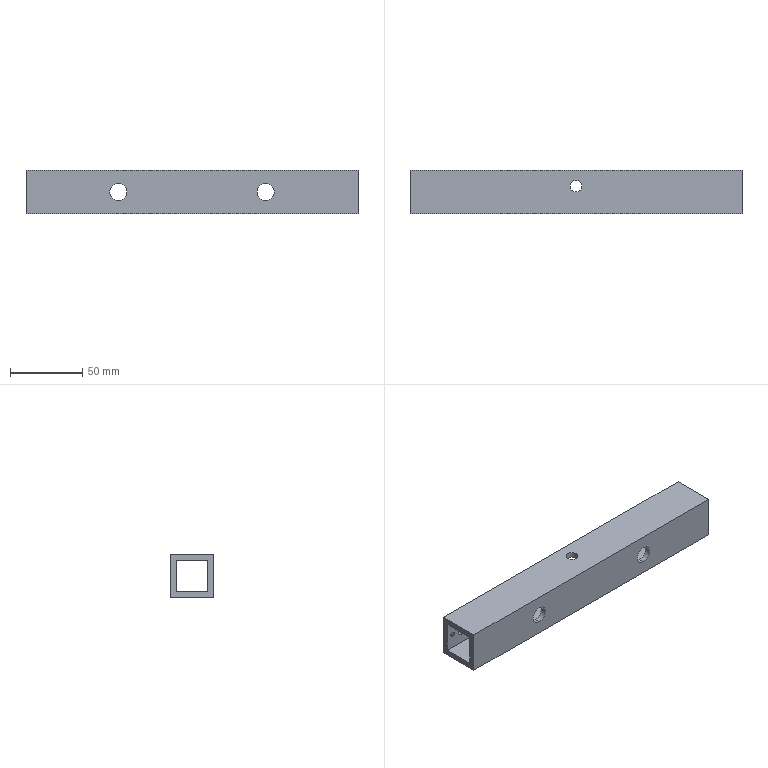Part | STEP file | Blade fixing rod | 1 solid | 37 faces | box 230 x 30 x 30 mm | volume 83181 mm3 | cylinder 24 | plane 13 | commonest cylinder face diameters 3.3 x8 4 x4 8 x4 9 x4 12 x4
STEP:
#1=CARTESIAN_POINT('',(-51.,4.,7.318));
#2=VERTEX_POINT('',#1);
#3=CARTESIAN_POINT('',(-51.,4.,-4.682));
#4=VERTEX_POINT('',#3);
#5=CARTESIAN_POINT('',(-51.,4.,1.318));
#6=DIRECTION('',(0.,-1.,0.));
#7=DIRECTION('',(0.,0.,-1.));
#8=AXIS2_PLACEMENT_3D('',#5,#6,#7);
#9=CIRCLE('',#8,6.);
#10=EDGE_CURVE('',#2,#4,#9,.T.);
#11=ORIENTED_EDGE('',*,*,#10,.F.);
#12=CARTESIAN_POINT('',(-51.,0.,7.318));
#13=VERTEX_POINT('',#12);
#14=CARTESIAN_POINT('',(-51.,0.,7.318));
#15=DIRECTION('',(0.,-1.,0.));
#16=VECTOR('',#15,1000.);
#17=LINE('',#14,#16);
#18=EDGE_CURVE('',#2,#13,#17,.T.);
#19=ORIENTED_EDGE('',*,*,#18,.T.);
#20=CARTESIAN_POINT('',(-51.,0.,-4.682));
#21=VERTEX_POINT('',#20);
#22=CARTESIAN_POINT('',(-51.,0.,1.318));
#23=DIRECTION('',(0.,-1.,0.));
#24=DIRECTION('',(0.,0.,-1.));
#25=AXIS2_PLACEMENT_3D('',#22,#23,#24);
#26=CIRCLE('',#25,6.);
#27=EDGE_CURVE('',#13,#21,#26,.T.);
#28=ORIENTED_EDGE('',*,*,#27,.T.);
#29=CARTESIAN_POINT('',(-51.,0.,-4.682));
#30=DIRECTION('',(0.,-1.,0.));
#31=VECTOR('',#30,1000.);
#32=LINE('',#29,#31);
#33=EDGE_CURVE('',#4,#21,#32,.T.);
#34=ORIENTED_EDGE('',*,*,#33,.F.);
#35=EDGE_LOOP('',(#11,#19,#28,#34));
#36=FACE_OUTER_BOUND('',#35,.T.);
#37=CARTESIAN_POINT('',(-51.,0.,1.318));
#38=DIRECTION('',(0.,-1.,0.));
#39=DIRECTION('',(0.,0.,-1.));
#40=AXIS2_PLACEMENT_3D('',#37,#38,#39);
#41=CYLINDRICAL_SURFACE('',#40,6.);
#42=ADVANCED_FACE('',(#36),#41,.F.);
#43=CARTESIAN_POINT('',(51.,4.,7.318));
#44=VERTEX_POINT('',#43);
#45=CARTESIAN_POINT('',(51.,4.,-4.682));
#46=VERTEX_POINT('',#45);
#47=CARTESIAN_POINT('',(51.,4.,1.318));
#48=DIRECTION('',(0.,-1.,0.));
#49=DIRECTION('',(0.,0.,-1.));
#50=AXIS2_PLACEMENT_3D('',#47,#48,#49);
#51=CIRCLE('',#50,6.);
#52=EDGE_CURVE('',#44,#46,#51,.T.);
#53=ORIENTED_EDGE('',*,*,#52,.F.);
#54=CARTESIAN_POINT('',(51.,0.,7.318));
#55=VERTEX_POINT('',#54);
#56=CARTESIAN_POINT('',(51.,0.,7.318));
#57=DIRECTION('',(0.,-1.,0.));
#58=VECTOR('',#57,1000.);
#59=LINE('',#56,#58);
#60=EDGE_CURVE('',#44,#55,#59,.T.);
#61=ORIENTED_EDGE('',*,*,#60,.T.);
#62=CARTESIAN_POINT('',(51.,0.,-4.682));
#63=VERTEX_POINT('',#62);
#64=CARTESIAN_POINT('',(51.,0.,1.318));
#65=DIRECTION('',(0.,-1.,0.));
#66=DIRECTION('',(0.,0.,-1.));
#67=AXIS2_PLACEMENT_3D('',#64,#65,#66);
#68=CIRCLE('',#67,6.);
#69=EDGE_CURVE('',#55,#63,#68,.T.);
#70=ORIENTED_EDGE('',*,*,#69,.T.);
#71=CARTESIAN_POINT('',(51.,0.,-4.682));
#72=DIRECTION('',(0.,-1.,0.));
#73=VECTOR('',#72,1000.);
#74=LINE('',#71,#73);
#75=EDGE_CURVE('',#46,#63,#74,.T.);
#76=ORIENTED_EDGE('',*,*,#75,.F.);
#77=EDGE_LOOP('',(#53,#61,#70,#76));
#78=FACE_OUTER_BOUND('',#77,.T.);
#79=CARTESIAN_POINT('',(51.,0.,1.318));
#80=DIRECTION('',(0.,-1.,0.));
#81=DIRECTION('',(0.,0.,-1.));
#82=AXIS2_PLACEMENT_3D('',#79,#80,#81);
#83=CYLINDRICAL_SURFACE('',#82,6.);
#84=ADVANCED_FACE('',(#78),#83,.F.);
#85=CARTESIAN_POINT('',(110.,26.,-0.3322));
#86=VERTEX_POINT('',#85);
#87=CARTESIAN_POINT('',(110.,26.,2.968));
#88=VERTEX_POINT('',#87);
#89=CARTESIAN_POINT('',(110.,26.,1.318));
#90=DIRECTION('',(0.,1.,0.));
#91=DIRECTION('',(0.,0.,1.));
#92=AXIS2_PLACEMENT_3D('',#89,#90,#91);
#93=CIRCLE('',#92,1.65);
#94=EDGE_CURVE('',#86,#88,#93,.T.);
#95=ORIENTED_EDGE('',*,*,#94,.F.);
#96=CARTESIAN_POINT('',(110.,30.,-0.3322));
#97=VERTEX_POINT('',#96);
#98=CARTESIAN_POINT('',(110.,30.,-0.3322));
#99=DIRECTION('',(0.,1.,0.));
#100=VECTOR('',#99,1000.);
#101=LINE('',#98,#100);
#102=EDGE_CURVE('',#86,#97,#101,.T.);
#103=ORIENTED_EDGE('',*,*,#102,.T.);
#104=CARTESIAN_POINT('',(110.,30.,2.968));
#105=VERTEX_POINT('',#104);
#106=CARTESIAN_POINT('',(110.,30.,1.318));
#107=DIRECTION('',(0.,1.,0.));
#108=DIRECTION('',(0.,0.,1.));
#109=AXIS2_PLACEMENT_3D('',#106,#107,#108);
#110=CIRCLE('',#109,1.65);
#111=EDGE_CURVE('',#97,#105,#110,.T.);
#112=ORIENTED_EDGE('',*,*,#111,.T.);
#113=CARTESIAN_POINT('',(110.,30.,2.968));
#114=DIRECTION('',(0.,1.,0.));
#115=VECTOR('',#114,1000.);
#116=LINE('',#113,#115);
#117=EDGE_CURVE('',#88,#105,#116,.T.);
#118=ORIENTED_EDGE('',*,*,#117,.F.);
#119=EDGE_LOOP('',(#95,#103,#112,#118));
#120=FACE_OUTER_BOUND('',#119,.T.);
#121=CARTESIAN_POINT('',(110.,30.,1.318));
#122=DIRECTION('',(0.,1.,0.));
#123=DIRECTION('',(0.,0.,1.));
#124=AXIS2_PLACEMENT_3D('',#121,#122,#123);
#125=CYLINDRICAL_SURFACE('',#124,1.65);
#126=ADVANCED_FACE('',(#120),#125,.F.);
#127=CARTESIAN_POINT('',(90.,26.,-0.3322));
#128=VERTEX_POINT('',#127);
#129=CARTESIAN_POINT('',(90.,26.,2.968));
#130=VERTEX_POINT('',#129);
#131=CARTESIAN_POINT('',(90.,26.,1.318));
#132=DIRECTION('',(0.,1.,0.));
#133=DIRECTION('',(0.,0.,1.));
#134=AXIS2_PLACEMENT_3D('',#131,#132,#133);
#135=CIRCLE('',#134,1.65);
#136=EDGE_CURVE('',#128,#130,#135,.T.);
#137=ORIENTED_EDGE('',*,*,#136,.F.);
#138=CARTESIAN_POINT('',(90.,30.,-0.3322));
#139=VERTEX_POINT('',#138);
#140=CARTESIAN_POINT('',(90.,30.,-0.3322));
#141=DIRECTION('',(0.,1.,0.));
#142=VECTOR('',#141,1000.);
#143=LINE('',#140,#142);
#144=EDGE_CURVE('',#128,#139,#143,.T.);
#145=ORIENTED_EDGE('',*,*,#144,.T.);
#146=CARTESIAN_POINT('',(90.,30.,2.968));
#147=VERTEX_POINT('',#146);
#148=CARTESIAN_POINT('',(90.,30.,1.318));
#149=DIRECTION('',(0.,1.,0.));
#150=DIRECTION('',(0.,0.,1.));
#151=AXIS2_PLACEMENT_3D('',#148,#149,#150);
#152=CIRCLE('',#151,1.65);
#153=EDGE_CURVE('',#139,#147,#152,.T.);
#154=ORIENTED_EDGE('',*,*,#153,.T.);
#155=CARTESIAN_POINT('',(90.,30.,2.968));
#156=DIRECTION('',(0.,1.,0.));
#157=VECTOR('',#156,1000.);
#158=LINE('',#155,#157);
#159=EDGE_CURVE('',#130,#147,#158,.T.);
#160=ORIENTED_EDGE('',*,*,#159,.F.);
#161=EDGE_LOOP('',(#137,#145,#154,#160));
#162=FACE_OUTER_BOUND('',#161,.T.);
#163=CARTESIAN_POINT('',(90.,30.,1.318));
#164=DIRECTION('',(0.,1.,0.));
#165=DIRECTION('',(0.,0.,1.));
#166=AXIS2_PLACEMENT_3D('',#163,#164,#165);
#167=CYLINDRICAL_SURFACE('',#166,1.65);
#168=ADVANCED_FACE('',(#162),#167,.F.);
#169=CARTESIAN_POINT('',(-110.,26.,-0.3322));
#170=VERTEX_POINT('',#169);
#171=CARTESIAN_POINT('',(-110.,26.,2.968));
#172=VERTEX_POINT('',#171);
#173=CARTESIAN_POINT('',(-110.,26.,1.318));
#174=DIRECTION('',(0.,1.,0.));
#175=DIRECTION('',(0.,0.,1.));
#176=AXIS2_PLACEMENT_3D('',#173,#174,#175);
#177=CIRCLE('',#176,1.65);
#178=EDGE_CURVE('',#170,#172,#177,.T.);
#179=ORIENTED_EDGE('',*,*,#178,.F.);
#180=CARTESIAN_POINT('',(-110.,30.,-0.3322));
#181=VERTEX_POINT('',#180);
#182=CARTESIAN_POINT('',(-110.,30.,-0.3322));
#183=DIRECTION('',(0.,1.,0.));
#184=VECTOR('',#183,1000.);
#185=LINE('',#182,#184);
#186=EDGE_CURVE('',#170,#181,#185,.T.);
#187=ORIENTED_EDGE('',*,*,#186,.T.);
#188=CARTESIAN_POINT('',(-110.,30.,2.968));
#189=VERTEX_POINT('',#188);
#190=CARTESIAN_POINT('',(-110.,30.,1.318));
#191=DIRECTION('',(0.,1.,0.));
#192=DIRECTION('',(0.,0.,1.));
#193=AXIS2_PLACEMENT_3D('',#190,#191,#192);
#194=CIRCLE('',#193,1.65);
#195=EDGE_CURVE('',#181,#189,#194,.T.);
#196=ORIENTED_EDGE('',*,*,#195,.T.);
#197=CARTESIAN_POINT('',(-110.,30.,2.968));
#198=DIRECTION('',(0.,1.,0.));
#199=VECTOR('',#198,1000.);
#200=LINE('',#197,#199);
#201=EDGE_CURVE('',#172,#189,#200,.T.);
#202=ORIENTED_EDGE('',*,*,#201,.F.);
#203=EDGE_LOOP('',(#179,#187,#196,#202));
#204=FACE_OUTER_BOUND('',#203,.T.);
#205=CARTESIAN_POINT('',(-110.,30.,1.318));
#206=DIRECTION('',(0.,1.,0.));
#207=DIRECTION('',(0.,0.,1.));
#208=AXIS2_PLACEMENT_3D('',#205,#206,#207);
#209=CYLINDRICAL_SURFACE('',#208,1.65);
#210=ADVANCED_FACE('',(#204),#209,.F.);
#211=CARTESIAN_POINT('',(-90.,26.,-0.3322));
#212=VERTEX_POINT('',#211);
#213=CARTESIAN_POINT('',(-90.,26.,2.968));
#214=VERTEX_POINT('',#213);
#215=CARTESIAN_POINT('',(-90.,26.,1.318));
#216=DIRECTION('',(0.,1.,0.));
#217=DIRECTION('',(0.,0.,1.));
#218=AXIS2_PLACEMENT_3D('',#215,#216,#217);
#219=CIRCLE('',#218,1.65);
#220=EDGE_CURVE('',#212,#214,#219,.T.);
#221=ORIENTED_EDGE('',*,*,#220,.F.);
#222=CARTESIAN_POINT('',(-90.,30.,-0.3322));
#223=VERTEX_POINT('',#222);
#224=CARTESIAN_POINT('',(-90.,30.,-0.3322));
#225=DIRECTION('',(0.,1.,0.));
#226=VECTOR('',#225,1000.);
#227=LINE('',#224,#226);
#228=EDGE_CURVE('',#212,#223,#227,.T.);
#229=ORIENTED_EDGE('',*,*,#228,.T.);
#230=CARTESIAN_POINT('',(-90.,30.,2.968));
#231=VERTEX_POINT('',#230);
#232=CARTESIAN_POINT('',(-90.,30.,1.318));
#233=DIRECTION('',(0.,1.,0.));
#234=DIRECTION('',(0.,0.,1.));
#235=AXIS2_PLACEMENT_3D('',#232,#233,#234);
#236=CIRCLE('',#235,1.65);
#237=EDGE_CURVE('',#223,#231,#236,.T.);
#238=ORIENTED_EDGE('',*,*,#237,.T.);
#239=CARTESIAN_POINT('',(-90.,30.,2.968));
#240=DIRECTION('',(0.,1.,0.));
#241=VECTOR('',#240,1000.);
#242=LINE('',#239,#241);
#243=EDGE_CURVE('',#214,#231,#242,.T.);
#244=ORIENTED_EDGE('',*,*,#243,.F.);
#245=EDGE_LOOP('',(#221,#229,#238,#244));
#246=FACE_OUTER_BOUND('',#245,.T.);
#247=CARTESIAN_POINT('',(-90.,30.,1.318));
#248=DIRECTION('',(0.,1.,0.));
#249=DIRECTION('',(0.,0.,1.));
#250=AXIS2_PLACEMENT_3D('',#247,#248,#249);
#251=CYLINDRICAL_SURFACE('',#250,1.65);
#252=ADVANCED_FACE('',(#246),#251,.F.);
#253=CARTESIAN_POINT('',(100.,26.,-3.182));
#254=VERTEX_POINT('',#253);
#255=CARTESIAN_POINT('',(100.,26.,5.818));
#256=VERTEX_POINT('',#255);
#257=CARTESIAN_POINT('',(100.,26.,1.318));
#258=DIRECTION('',(0.,1.,0.));
#259=DIRECTION('',(0.,0.,1.));
#260=AXIS2_PLACEMENT_3D('',#257,#258,#259);
#261=CIRCLE('',#260,4.5);
#262=EDGE_CURVE('',#254,#256,#261,.T.);
#263=ORIENTED_EDGE('',*,*,#262,.F.);
#264=CARTESIAN_POINT('',(100.,30.,-3.182));
#265=VERTEX_POINT('',#264);
#266=CARTESIAN_POINT('',(100.,20.,-3.182));
#267=DIRECTION('',(0.,1.,0.));
#268=VECTOR('',#267,1000.);
#269=LINE('',#266,#268);
#270=EDGE_CURVE('',#254,#265,#269,.T.);
#271=ORIENTED_EDGE('',*,*,#270,.T.);
#272=CARTESIAN_POINT('',(100.,30.,5.818));
#273=VERTEX_POINT('',#272);
#274=CARTESIAN_POINT('',(100.,30.,1.318));
#275=DIRECTION('',(0.,1.,0.));
#276=DIRECTION('',(0.,0.,-1.));
#277=AXIS2_PLACEMENT_3D('',#274,#275,#276);
#278=CIRCLE('',#277,4.5);
#279=EDGE_CURVE('',#265,#273,#278,.T.);
#280=ORIENTED_EDGE('',*,*,#279,.T.);
#281=CARTESIAN_POINT('',(100.,20.,5.818));
#282=DIRECTION('',(0.,1.,0.));
#283=VECTOR('',#282,1000.);
#284=LINE('',#281,#283);
#285=EDGE_CURVE('',#256,#273,#284,.T.);
#286=ORIENTED_EDGE('',*,*,#285,.F.);
#287=EDGE_LOOP('',(#263,#271,#280,#286));
#288=FACE_OUTER_BOUND('',#287,.T.);
#289=CARTESIAN_POINT('',(100.,20.,1.318));
#290=DIRECTION('',(0.,1.,0.));
#291=DIRECTION('',(0.,0.,1.));
#292=AXIS2_PLACEMENT_3D('',#289,#290,#291);
#293=CYLINDRICAL_SURFACE('',#292,4.5);
#294=ADVANCED_FACE('',(#288),#293,.F.);
#295=CARTESIAN_POINT('',(-100.,26.,-3.182));
#296=VERTEX_POINT('',#295);
#297=CARTESIAN_POINT('',(-100.,26.,5.818));
#298=VERTEX_POINT('',#297);
#299=CARTESIAN_POINT('',(-100.,26.,1.318));
#300=DIRECTION('',(0.,1.,0.));
#301=DIRECTION('',(0.,0.,1.));
#302=AXIS2_PLACEMENT_3D('',#299,#300,#301);
#303=CIRCLE('',#302,4.5);
#304=EDGE_CURVE('',#296,#298,#303,.T.);
#305=ORIENTED_EDGE('',*,*,#304,.F.);
#306=CARTESIAN_POINT('',(-100.,30.,-3.182));
#307=VERTEX_POINT('',#306);
#308=CARTESIAN_POINT('',(-100.,20.,-3.182));
#309=DIRECTION('',(0.,1.,0.));
#310=VECTOR('',#309,1000.);
#311=LINE('',#308,#310);
#312=EDGE_CURVE('',#296,#307,#311,.T.);
#313=ORIENTED_EDGE('',*,*,#312,.T.);
#314=CARTESIAN_POINT('',(-100.,30.,5.818));
#315=VERTEX_POINT('',#314);
#316=CARTESIAN_POINT('',(-100.,30.,1.318));
#317=DIRECTION('',(0.,1.,0.));
#318=DIRECTION('',(0.,0.,1.));
#319=AXIS2_PLACEMENT_3D('',#316,#317,#318);
#320=CIRCLE('',#319,4.5);
#321=EDGE_CURVE('',#307,#315,#320,.T.);
#322=ORIENTED_EDGE('',*,*,#321,.T.);
#323=CARTESIAN_POINT('',(-100.,20.,5.818));
#324=DIRECTION('',(0.,1.,0.));
#325=VECTOR('',#324,1000.);
#326=LINE('',#323,#325);
#327=EDGE_CURVE('',#298,#315,#326,.T.);
#328=ORIENTED_EDGE('',*,*,#327,.F.);
#329=EDGE_LOOP('',(#305,#313,#322,#328));
#330=FACE_OUTER_BOUND('',#329,.T.);
#331=CARTESIAN_POINT('',(-100.,20.,1.318));
#332=DIRECTION('',(0.,1.,0.));
#333=DIRECTION('',(0.,0.,1.));
#334=AXIS2_PLACEMENT_3D('',#331,#332,#333);
#335=CYLINDRICAL_SURFACE('',#334,4.5);
#336=ADVANCED_FACE('',(#330),#335,.F.);
#337=CARTESIAN_POINT('',(4.,19.,16.318));
#338=VERTEX_POINT('',#337);
#339=CARTESIAN_POINT('',(-4.,19.,16.318));
#340=VERTEX_POINT('',#339);
#341=CARTESIAN_POINT('',(0.,19.,16.318));
#342=DIRECTION('',(0.,0.,-1.));
#343=DIRECTION('',(-1.,0.,0.));
#344=AXIS2_PLACEMENT_3D('',#341,#342,#343);
#345=CIRCLE('',#344,4.);
#346=EDGE_CURVE('',#338,#340,#345,.T.);
#347=ORIENTED_EDGE('',*,*,#346,.F.);
#348=CARTESIAN_POINT('',(4.,19.,12.318));
#349=VERTEX_POINT('',#348);
#350=CARTESIAN_POINT('',(4.,19.,16.318));
#351=DIRECTION('',(0.,0.,-1.));
#352=VECTOR('',#351,1000.);
#353=LINE('',#350,#352);
#354=EDGE_CURVE('',#338,#349,#353,.T.);
#355=ORIENTED_EDGE('',*,*,#354,.T.);
#356=CARTESIAN_POINT('',(-4.,19.,12.318));
#357=VERTEX_POINT('',#356);
#358=CARTESIAN_POINT('',(0.,19.,12.318));
#359=DIRECTION('',(0.,0.,1.));
#360=DIRECTION('',(1.,0.,0.));
#361=AXIS2_PLACEMENT_3D('',#358,#359,#360);
#362=CIRCLE('',#361,4.);
#363=EDGE_CURVE('',#357,#349,#362,.T.);
#364=ORIENTED_EDGE('',*,*,#363,.F.);
#365=CARTESIAN_POINT('',(-4.,19.,16.318));
#366=DIRECTION('',(0.,0.,-1.));
#367=VECTOR('',#366,1000.);
#368=LINE('',#365,#367);
#369=EDGE_CURVE('',#340,#357,#368,.T.);
#370=ORIENTED_EDGE('',*,*,#369,.F.);
#371=EDGE_LOOP('',(#347,#355,#364,#370));
#372=FACE_OUTER_BOUND('',#371,.T.);
#373=CARTESIAN_POINT('',(0.,19.,16.318));
#374=DIRECTION('',(0.,0.,-1.));
#375=DIRECTION('',(-1.,0.,0.));
#376=AXIS2_PLACEMENT_3D('',#373,#374,#375);
#377=CYLINDRICAL_SURFACE('',#376,4.);
#378=ADVANCED_FACE('',(#372),#377,.F.);
#379=CARTESIAN_POINT('',(4.,19.,-9.682));
#380=VERTEX_POINT('',#379);
#381=CARTESIAN_POINT('',(-4.,19.,-9.682));
#382=VERTEX_POINT('',#381);
#383=CARTESIAN_POINT('',(0.,19.,-9.682));
#384=DIRECTION('',(0.,0.,-1.));
#385=DIRECTION('',(-1.,0.,0.));
#386=AXIS2_PLACEMENT_3D('',#383,#384,#385);
#387=CIRCLE('',#386,4.);
#388=EDGE_CURVE('',#380,#382,#387,.T.);
#389=ORIENTED_EDGE('',*,*,#388,.F.);
#390=CARTESIAN_POINT('',(4.,19.,-13.682));
#391=VERTEX_POINT('',#390);
#392=CARTESIAN_POINT('',(4.,19.,16.318));
#393=DIRECTION('',(0.,0.,-1.));
#394=VECTOR('',#393,1000.);
#395=LINE('',#392,#394);
#396=EDGE_CURVE('',#380,#391,#395,.T.);
#397=ORIENTED_EDGE('',*,*,#396,.T.);
#398=CARTESIAN_POINT('',(-4.,19.,-13.682));
#399=VERTEX_POINT('',#398);
#400=CARTESIAN_POINT('',(0.,19.,-13.682));
#401=DIRECTION('',(0.,0.,-1.));
#402=DIRECTION('',(-1.,0.,0.));
#403=AXIS2_PLACEMENT_3D('',#400,#401,#402);
#404=CIRCLE('',#403,4.);
#405=EDGE_CURVE('',#391,#399,#404,.T.);
#406=ORIENTED_EDGE('',*,*,#405,.T.);
#407=CARTESIAN_POINT('',(-4.,19.,16.318));
#408=DIRECTION('',(0.,0.,-1.));
#409=VECTOR('',#408,1000.);
#410=LINE('',#407,#409);
#411=EDGE_CURVE('',#382,#399,#410,.T.);
#412=ORIENTED_EDGE('',*,*,#411,.F.);
#413=EDGE_LOOP('',(#389,#397,#406,#412));
#414=FACE_OUTER_BOUND('',#413,.T.);
#415=CARTESIAN_POINT('',(0.,19.,16.318));
#416=DIRECTION('',(0.,0.,-1.));
#417=DIRECTION('',(-1.,0.,0.));
#418=AXIS2_PLACEMENT_3D('',#415,#416,#417);
#419=CYLINDRICAL_SURFACE('',#418,4.);
#420=ADVANCED_FACE('',(#414),#419,.F.);
#421=CARTESIAN_POINT('',(110.,26.,1.318));
#422=DIRECTION('',(0.,1.,0.));
#423=DIRECTION('',(0.,0.,1.));
#424=AXIS2_PLACEMENT_3D('',#421,#422,#423);
#425=CIRCLE('',#424,1.65);
#426=EDGE_CURVE('',#88,#86,#425,.T.);
#427=ORIENTED_EDGE('',*,*,#426,.T.);
#428=ORIENTED_EDGE('',*,*,#94,.T.);
#429=EDGE_LOOP('',(#427,#428));
#430=FACE_BOUND('',#429,.T.);
#431=CARTESIAN_POINT('',(90.,26.,1.318));
#432=DIRECTION('',(0.,1.,0.));
#433=DIRECTION('',(0.,0.,1.));
#434=AXIS2_PLACEMENT_3D('',#431,#432,#433);
#435=CIRCLE('',#434,1.65);
#436=EDGE_CURVE('',#130,#128,#435,.T.);
#437=ORIENTED_EDGE('',*,*,#436,.T.);
#438=ORIENTED_EDGE('',*,*,#136,.T.);
#439=EDGE_LOOP('',(#437,#438));
#440=FACE_BOUND('',#439,.T.);
#441=CARTESIAN_POINT('',(100.,26.,1.318));
#442=DIRECTION('',(0.,1.,0.));
#443=DIRECTION('',(0.,0.,1.));
#444=AXIS2_PLACEMENT_3D('',#441,#442,#443);
#445=CIRCLE('',#444,4.5);
#446=EDGE_CURVE('',#256,#254,#445,.T.);
#447=ORIENTED_EDGE('',*,*,#446,.T.);
#448=ORIENTED_EDGE('',*,*,#262,.T.);
#449=EDGE_LOOP('',(#447,#448));
#450=FACE_BOUND('',#449,.T.);
#451=CARTESIAN_POINT('',(115.,26.,12.318));
#452=VERTEX_POINT('',#451);
#453=CARTESIAN_POINT('',(58.,26.,12.318));
#454=VERTEX_POINT('',#453);
#455=CARTESIAN_POINT('',(115.,26.,12.318));
#456=DIRECTION('',(-1.,0.,0.));
#457=VECTOR('',#456,1000.);
#458=LINE('',#455,#457);
#459=EDGE_CURVE('',#452,#454,#458,.T.);
#460=ORIENTED_EDGE('',*,*,#459,.T.);
#461=CARTESIAN_POINT('',(60.,26.,10.318));
#462=VERTEX_POINT('',#461);
#463=CARTESIAN_POINT('',(58.,26.,10.318));
#464=DIRECTION('',(0.,1.,0.));
#465=DIRECTION('',(0.,0.,1.));
#466=AXIS2_PLACEMENT_3D('',#463,#464,#465);
#467=CIRCLE('',#466,2.);
#468=EDGE_CURVE('',#454,#462,#467,.T.);
#469=ORIENTED_EDGE('',*,*,#468,.T.);
#470=CARTESIAN_POINT('',(60.,26.,-7.682));
#471=VERTEX_POINT('',#470);
#472=CARTESIAN_POINT('',(60.,26.,-9.682));
#473=DIRECTION('',(0.,0.,-1.));
#474=VECTOR('',#473,1000.);
#475=LINE('',#472,#474);
#476=EDGE_CURVE('',#462,#471,#475,.T.);
#477=ORIENTED_EDGE('',*,*,#476,.T.);
#478=CARTESIAN_POINT('',(58.,26.,-9.682));
#479=VERTEX_POINT('',#478);
#480=CARTESIAN_POINT('',(58.,26.,-7.682));
#481=DIRECTION('',(0.,1.,0.));
#482=DIRECTION('',(0.,0.,1.));
#483=AXIS2_PLACEMENT_3D('',#480,#481,#482);
#484=CIRCLE('',#483,2.);
#485=EDGE_CURVE('',#471,#479,#484,.T.);
#486=ORIENTED_EDGE('',*,*,#485,.T.);
#487=CARTESIAN_POINT('',(115.,26.,-9.682));
#488=VERTEX_POINT('',#487);
#489=CARTESIAN_POINT('',(115.,26.,-9.682));
#490=DIRECTION('',(-1.,0.,0.));
#491=VECTOR('',#490,1000.);
#492=LINE('',#489,#491);
#493=EDGE_CURVE('',#488,#479,#492,.T.);
#494=ORIENTED_EDGE('',*,*,#493,.F.);
#495=CARTESIAN_POINT('',(115.,26.,-9.682));
#496=DIRECTION('',(0.,0.,-1.));
#497=VECTOR('',#496,1000.);
#498=LINE('',#495,#497);
#499=EDGE_CURVE('',#452,#488,#498,.T.);
#500=ORIENTED_EDGE('',*,*,#499,.F.);
#501=EDGE_LOOP('',(#460,#469,#477,#486,#494,#500));
#502=FACE_OUTER_BOUND('',#501,.T.);
#503=CARTESIAN_POINT('',(115.,26.,-9.682));
#504=DIRECTION('',(0.,1.,0.));
#505=DIRECTION('',(0.,0.,1.));
#506=AXIS2_PLACEMENT_3D('',#503,#504,#505);
#507=PLANE('',#506);
#508=ADVANCED_FACE('',(#430,#440,#450,#502),#507,.F.);
#509=CARTESIAN_POINT('',(115.,4.,-9.682));
#510=VERTEX_POINT('',#509);
#511=CARTESIAN_POINT('',(115.,4.,12.318));
#512=VERTEX_POINT('',#511);
#513=CARTESIAN_POINT('',(115.,4.,-9.682));
#514=DIRECTION('',(0.,0.,1.));
#515=VECTOR('',#514,1000.);
#516=LINE('',#513,#515);
#517=EDGE_CURVE('',#510,#512,#516,.T.);
#518=ORIENTED_EDGE('',*,*,#517,.T.);
#519=CARTESIAN_POINT('',(115.,4.,12.318));
#520=DIRECTION('',(0.,1.,0.));
#521=VECTOR('',#520,1000.);
#522=LINE('',#519,#521);
#523=EDGE_CURVE('',#512,#452,#522,.T.);
#524=ORIENTED_EDGE('',*,*,#523,.T.);
#525=ORIENTED_EDGE('',*,*,#499,.T.);
#526=CARTESIAN_POINT('',(115.,4.,-9.682));
#527=DIRECTION('',(0.,-1.,0.));
#528=VECTOR('',#527,1000.);
#529=LINE('',#526,#528);
#530=EDGE_CURVE('',#488,#510,#529,.T.);
#531=ORIENTED_EDGE('',*,*,#530,.T.);
#532=EDGE_LOOP('',(#518,#524,#525,#531));
#533=FACE_BOUND('',#532,.T.);
#534=CARTESIAN_POINT('',(115.,0.,16.318));
#535=VERTEX_POINT('',#534);
#536=CARTESIAN_POINT('',(115.,0.,-13.682));
#537=VERTEX_POINT('',#536);
#538=CARTESIAN_POINT('',(115.,0.,16.318));
#539=DIRECTION('',(0.,0.,-1.));
#540=VECTOR('',#539,1000.);
#541=LINE('',#538,#540);
#542=EDGE_CURVE('',#535,#537,#541,.T.);
#543=ORIENTED_EDGE('',*,*,#542,.T.);
#544=CARTESIAN_POINT('',(115.,30.,-13.682));
#545=VERTEX_POINT('',#544);
#546=CARTESIAN_POINT('',(115.,30.,-13.682));
#547=DIRECTION('',(0.,-1.,0.));
#548=VECTOR('',#547,1000.);
#549=LINE('',#546,#548);
#550=EDGE_CURVE('',#545,#537,#549,.T.);
#551=ORIENTED_EDGE('',*,*,#550,.F.);
#552=CARTESIAN_POINT('',(115.,30.,16.318));
#553=VERTEX_POINT('',#552);
#554=CARTESIAN_POINT('',(115.,30.,16.318));
#555=DIRECTION('',(0.,0.,-1.));
#556=VECTOR('',#555,1000.);
#557=LINE('',#554,#556);
#558=EDGE_CURVE('',#553,#545,#557,.T.);
#559=ORIENTED_EDGE('',*,*,#558,.F.);
#560=CARTESIAN_POINT('',(115.,30.,16.318));
#561=DIRECTION('',(0.,-1.,0.));
#562=VECTOR('',#561,1000.);
#563=LINE('',#560,#562);
#564=EDGE_CURVE('',#553,#535,#563,.T.);
#565=ORIENTED_EDGE('',*,*,#564,.T.);
#566=EDGE_LOOP('',(#543,#551,#559,#565));
#567=FACE_OUTER_BOUND('',#566,.T.);
#568=CARTESIAN_POINT('',(115.,30.,16.318));
#569=DIRECTION('',(-1.,0.,0.));
#570=DIRECTION('',(0.,0.,1.));
#571=AXIS2_PLACEMENT_3D('',#568,#569,#570);
#572=PLANE('',#571);
#573=ADVANCED_FACE('',(#533,#567),#572,.F.);
#574=CARTESIAN_POINT('',(0.,19.,-13.682));
#575=DIRECTION('',(0.,0.,-1.));
#576=DIRECTION('',(-1.,0.,0.));
#577=AXIS2_PLACEMENT_3D('',#574,#575,#576);
#578=CIRCLE('',#577,4.);
#579=EDGE_CURVE('',#399,#391,#578,.T.);
#580=ORIENTED_EDGE('',*,*,#579,.F.);
#581=ORIENTED_EDGE('',*,*,#405,.F.);
#582=EDGE_LOOP('',(#580,#581));
#583=FACE_BOUND('',#582,.T.);
#584=CARTESIAN_POINT('',(-115.,0.,-13.682));
#585=VERTEX_POINT('',#584);
#586=CARTESIAN_POINT('',(-115.,0.,-13.682));
#587=DIRECTION('',(-1.,0.,0.));
#588=VECTOR('',#587,1000.);
#589=LINE('',#586,#588);
#590=EDGE_CURVE('',#537,#585,#589,.T.);
#591=ORIENTED_EDGE('',*,*,#590,.T.);
#592=CARTESIAN_POINT('',(-115.,30.,-13.682));
#593=VERTEX_POINT('',#592);
#594=CARTESIAN_POINT('',(-115.,30.,-13.682));
#595=DIRECTION('',(0.,-1.,0.));
#596=VECTOR('',#595,1000.);
#597=LINE('',#594,#596);
#598=EDGE_CURVE('',#593,#585,#597,.T.);
#599=ORIENTED_EDGE('',*,*,#598,.F.);
#600=CARTESIAN_POINT('',(-115.,30.,-13.682));
#601=DIRECTION('',(-1.,0.,0.));
#602=VECTOR('',#601,1000.);
#603=LINE('',#600,#602);
#604=EDGE_CURVE('',#545,#593,#603,.T.);
#605=ORIENTED_EDGE('',*,*,#604,.F.);
#606=ORIENTED_EDGE('',*,*,#550,.T.);
#607=EDGE_LOOP('',(#591,#599,#605,#606));
#608=FACE_OUTER_BOUND('',#607,.T.);
#609=CARTESIAN_POINT('',(-115.,30.,-13.682));
#610=DIRECTION('',(0.,0.,1.));
#611=DIRECTION('',(1.,0.,0.));
#612=AXIS2_PLACEMENT_3D('',#609,#610,#611);
#613=PLANE('',#612);
#614=ADVANCED_FACE('',(#583,#608),#613,.F.);
#615=CARTESIAN_POINT('',(-115.,26.,12.318));
#616=VERTEX_POINT('',#615);
#617=CARTESIAN_POINT('',(-115.,26.,-9.682));
#618=VERTEX_POINT('',#617);
#619=CARTESIAN_POINT('',(-115.,26.,-9.682));
#620=DIRECTION('',(0.,0.,-1.));
#621=VECTOR('',#620,1000.);
#622=LINE('',#619,#621);
#623=EDGE_CURVE('',#616,#618,#622,.T.);
#624=ORIENTED_EDGE('',*,*,#623,.F.);
#625=CARTESIAN_POINT('',(-115.,4.,12.318));
#626=VERTEX_POINT('',#625);
#627=CARTESIAN_POINT('',(-115.,4.,12.318));
#628=DIRECTION('',(0.,1.,0.));
#629=VECTOR('',#628,1000.);
#630=LINE('',#627,#629);
#631=EDGE_CURVE('',#626,#616,#630,.T.);
#632=ORIENTED_EDGE('',*,*,#631,.F.);
#633=CARTESIAN_POINT('',(-115.,4.,-9.682));
#634=VERTEX_POINT('',#633);
#635=CARTESIAN_POINT('',(-115.,4.,-9.682));
#636=DIRECTION('',(0.,0.,1.));
#637=VECTOR('',#636,1000.);
#638=LINE('',#635,#637);
#639=EDGE_CURVE('',#634,#626,#638,.T.);
#640=ORIENTED_EDGE('',*,*,#639,.F.);
#641=CARTESIAN_POINT('',(-115.,4.,-9.682));
#642=DIRECTION('',(0.,-1.,0.));
#643=VECTOR('',#642,1000.);
#644=LINE('',#641,#643);
#645=EDGE_CURVE('',#618,#634,#644,.T.);
#646=ORIENTED_EDGE('',*,*,#645,.F.);
#647=EDGE_LOOP('',(#624,#632,#640,#646));
#648=FACE_BOUND('',#647,.T.);
#649=CARTESIAN_POINT('',(-115.,0.,16.318));
#650=VERTEX_POINT('',#649);
#651=CARTESIAN_POINT('',(-115.,0.,16.318));
#652=DIRECTION('',(0.,0.,1.));
#653=VECTOR('',#652,1000.);
#654=LINE('',#651,#653);
#655=EDGE_CURVE('',#585,#650,#654,.T.);
#656=ORIENTED_EDGE('',*,*,#655,.T.);
#657=CARTESIAN_POINT('',(-115.,30.,16.318));
#658=VERTEX_POINT('',#657);
#659=CARTESIAN_POINT('',(-115.,30.,16.318));
#660=DIRECTION('',(0.,-1.,0.));
#661=VECTOR('',#660,1000.);
#662=LINE('',#659,#661);
#663=EDGE_CURVE('',#658,#650,#662,.T.);
#664=ORIENTED_EDGE('',*,*,#663,.F.);
#665=CARTESIAN_POINT('',(-115.,30.,16.318));
#666=DIRECTION('',(0.,0.,1.));
#667=VECTOR('',#666,1000.);
#668=LINE('',#665,#667);
#669=EDGE_CURVE('',#593,#658,#668,.T.);
#670=ORIENTED_EDGE('',*,*,#669,.F.);
#671=ORIENTED_EDGE('',*,*,#598,.T.);
#672=EDGE_LOOP('',(#656,#664,#670,#671));
#673=FACE_OUTER_BOUND('',#672,.T.);
#674=CARTESIAN_POINT('',(-115.,30.,16.318));
#675=DIRECTION('',(1.,0.,0.));
#676=DIRECTION('',(0.,0.,-1.));
#677=AXIS2_PLACEMENT_3D('',#674,#675,#676);
#678=PLANE('',#677);
#679=ADVANCED_FACE('',(#648,#673),#678,.F.);
#680=CARTESIAN_POINT('',(0.,19.,16.318));
#681=DIRECTION('',(0.,0.,-1.));
#682=DIRECTION('',(-1.,0.,0.));
#683=AXIS2_PLACEMENT_3D('',#680,#681,#682);
#684=CIRCLE('',#683,4.);
#685=EDGE_CURVE('',#340,#338,#684,.T.);
#686=ORIENTED_EDGE('',*,*,#685,.T.);
#687=ORIENTED_EDGE('',*,*,#346,.T.);
#688=EDGE_LOOP('',(#686,#687));
#689=FACE_BOUND('',#688,.T.);
#690=CARTESIAN_POINT('',(-115.,0.,16.318));
#691=DIRECTION('',(1.,0.,0.));
#692=VECTOR('',#691,1000.);
#693=LINE('',#690,#692);
#694=EDGE_CURVE('',#650,#535,#693,.T.);
#695=ORIENTED_EDGE('',*,*,#694,.T.);
#696=ORIENTED_EDGE('',*,*,#564,.F.);
#697=CARTESIAN_POINT('',(-115.,30.,16.318));
#698=DIRECTION('',(1.,0.,0.));
#699=VECTOR('',#698,1000.);
#700=LINE('',#697,#699);
#701=EDGE_CURVE('',#658,#553,#700,.T.);
#702=ORIENTED_EDGE('',*,*,#701,.F.);
#703=ORIENTED_EDGE('',*,*,#663,.T.);
#704=EDGE_LOOP('',(#695,#696,#702,#703));
#705=FACE_OUTER_BOUND('',#704,.T.);
#706=CARTESIAN_POINT('',(-115.,30.,16.318));
#707=DIRECTION('',(0.,0.,-1.));
#708=DIRECTION('',(-1.,0.,0.));
#709=AXIS2_PLACEMENT_3D('',#706,#707,#708);
#710=PLANE('',#709);
#711=ADVANCED_FACE('',(#689,#705),#710,.F.);
#712=CARTESIAN_POINT('',(110.,30.,1.318));
#713=DIRECTION('',(0.,1.,0.));
#714=DIRECTION('',(0.,0.,1.));
#715=AXIS2_PLACEMENT_3D('',#712,#713,#714);
#716=CIRCLE('',#715,1.65);
#717=EDGE_CURVE('',#105,#97,#716,.T.);
#718=ORIENTED_EDGE('',*,*,#717,.F.);
#719=ORIENTED_EDGE('',*,*,#111,.F.);
#720=EDGE_LOOP('',(#718,#719));
#721=FACE_BOUND('',#720,.T.);
#722=CARTESIAN_POINT('',(90.,30.,1.318));
#723=DIRECTION('',(0.,1.,0.));
#724=DIRECTION('',(0.,0.,1.));
#725=AXIS2_PLACEMENT_3D('',#722,#723,#724);
#726=CIRCLE('',#725,1.65);
#727=EDGE_CURVE('',#147,#139,#726,.T.);
#728=ORIENTED_EDGE('',*,*,#727,.F.);
#729=ORIENTED_EDGE('',*,*,#153,.F.);
#730=EDGE_LOOP('',(#728,#729));
#731=FACE_BOUND('',#730,.T.);
#732=CARTESIAN_POINT('',(-110.,30.,1.318));
#733=DIRECTION('',(0.,1.,0.));
#734=DIRECTION('',(0.,0.,1.));
#735=AXIS2_PLACEMENT_3D('',#732,#733,#734);
#736=CIRCLE('',#735,1.65);
#737=EDGE_CURVE('',#189,#181,#736,.T.);
#738=ORIENTED_EDGE('',*,*,#737,.F.);
#739=ORIENTED_EDGE('',*,*,#195,.F.);
#740=EDGE_LOOP('',(#738,#739));
#741=FACE_BOUND('',#740,.T.);
#742=CARTESIAN_POINT('',(-90.,30.,1.318));
#743=DIRECTION('',(0.,1.,0.));
#744=DIRECTION('',(0.,0.,1.));
#745=AXIS2_PLACEMENT_3D('',#742,#743,#744);
#746=CIRCLE('',#745,1.65);
#747=EDGE_CURVE('',#231,#223,#746,.T.);
#748=ORIENTED_EDGE('',*,*,#747,.F.);
#749=ORIENTED_EDGE('',*,*,#237,.F.);
#750=EDGE_LOOP('',(#748,#749));
#751=FACE_BOUND('',#750,.T.);
#752=CARTESIAN_POINT('',(100.,30.,1.318));
#753=DIRECTION('',(0.,1.,0.));
#754=DIRECTION('',(0.,0.,-1.));
#755=AXIS2_PLACEMENT_3D('',#752,#753,#754);
#756=CIRCLE('',#755,4.5);
#757=EDGE_CURVE('',#273,#265,#756,.T.);
#758=ORIENTED_EDGE('',*,*,#757,.F.);
#759=ORIENTED_EDGE('',*,*,#279,.F.);
#760=EDGE_LOOP('',(#758,#759));
#761=FACE_BOUND('',#760,.T.);
#762=CARTESIAN_POINT('',(-100.,30.,1.318));
#763=DIRECTION('',(0.,1.,0.));
#764=DIRECTION('',(0.,0.,1.));
#765=AXIS2_PLACEMENT_3D('',#762,#763,#764);
#766=CIRCLE('',#765,4.5);
#767=EDGE_CURVE('',#315,#307,#766,.T.);
#768=ORIENTED_EDGE('',*,*,#767,.F.);
#769=ORIENTED_EDGE('',*,*,#321,.F.);
#770=EDGE_LOOP('',(#768,#769));
#771=FACE_BOUND('',#770,.T.);
#772=CARTESIAN_POINT('',(58.,30.,-9.682));
#773=VERTEX_POINT('',#772);
#774=CARTESIAN_POINT('',(-58.,30.,-9.682));
#775=VERTEX_POINT('',#774);
#776=CARTESIAN_POINT('',(-60.,30.,-9.682));
#777=DIRECTION('',(-1.,0.,0.));
#778=VECTOR('',#777,1000.);
#779=LINE('',#776,#778);
#780=EDGE_CURVE('',#773,#775,#779,.T.);
#781=ORIENTED_EDGE('',*,*,#780,.F.);
#782=CARTESIAN_POINT('',(60.,30.,-7.682));
#783=VERTEX_POINT('',#782);
#784=CARTESIAN_POINT('',(58.,30.,-7.682));
#785=DIRECTION('',(0.,-1.,0.));
#786=DIRECTION('',(0.,0.,-1.));
#787=AXIS2_PLACEMENT_3D('',#784,#785,#786);
#788=CIRCLE('',#787,2.);
#789=EDGE_CURVE('',#773,#783,#788,.T.);
#790=ORIENTED_EDGE('',*,*,#789,.T.);
#791=CARTESIAN_POINT('',(60.,30.,10.318));
#792=VERTEX_POINT('',#791);
#793=CARTESIAN_POINT('',(60.,30.,12.318));
#794=DIRECTION('',(0.,0.,-1.));
#795=VECTOR('',#794,1000.);
#796=LINE('',#793,#795);
#797=EDGE_CURVE('',#792,#783,#796,.T.);
#798=ORIENTED_EDGE('',*,*,#797,.F.);
#799=CARTESIAN_POINT('',(58.,30.,12.318));
#800=VERTEX_POINT('',#799);
#801=CARTESIAN_POINT('',(58.,30.,10.318));
#802=DIRECTION('',(0.,-1.,0.));
#803=DIRECTION('',(0.,0.,-1.));
#804=AXIS2_PLACEMENT_3D('',#801,#802,#803);
#805=CIRCLE('',#804,2.);
#806=EDGE_CURVE('',#792,#800,#805,.T.);
#807=ORIENTED_EDGE('',*,*,#806,.T.);
#808=CARTESIAN_POINT('',(-58.,30.,12.318));
#809=VERTEX_POINT('',#808);
#810=CARTESIAN_POINT('',(-60.,30.,12.318));
#811=DIRECTION('',(1.,0.,0.));
#812=VECTOR('',#811,1000.);
#813=LINE('',#810,#812);
#814=EDGE_CURVE('',#809,#800,#813,.T.);
#815=ORIENTED_EDGE('',*,*,#814,.F.);
#816=CARTESIAN_POINT('',(-60.,30.,10.318));
#817=VERTEX_POINT('',#816);
#818=CARTESIAN_POINT('',(-58.,30.,10.318));
#819=DIRECTION('',(0.,-1.,0.));
#820=DIRECTION('',(0.,0.,-1.));
#821=AXIS2_PLACEMENT_3D('',#818,#819,#820);
#822=CIRCLE('',#821,2.);
#823=EDGE_CURVE('',#809,#817,#822,.T.);
#824=ORIENTED_EDGE('',*,*,#823,.T.);
#825=CARTESIAN_POINT('',(-60.,30.,-7.682));
#826=VERTEX_POINT('',#825);
#827=CARTESIAN_POINT('',(-60.,30.,12.318));
#828=DIRECTION('',(0.,0.,1.));
#829=VECTOR('',#828,1000.);
#830=LINE('',#827,#829);
#831=EDGE_CURVE('',#826,#817,#830,.T.);
#832=ORIENTED_EDGE('',*,*,#831,.F.);
#833=CARTESIAN_POINT('',(-58.,30.,-7.682));
#834=DIRECTION('',(0.,-1.,0.));
#835=DIRECTION('',(0.,0.,-1.));
#836=AXIS2_PLACEMENT_3D('',#833,#834,#835);
#837=CIRCLE('',#836,2.);
#838=EDGE_CURVE('',#826,#775,#837,.T.);
#839=ORIENTED_EDGE('',*,*,#838,.T.);
#840=EDGE_LOOP('',(#781,#790,#798,#807,#815,#824,#832,#839));
#841=FACE_BOUND('',#840,.T.);
#842=ORIENTED_EDGE('',*,*,#558,.T.);
#843=ORIENTED_EDGE('',*,*,#604,.T.);
#844=ORIENTED_EDGE('',*,*,#669,.T.);
#845=ORIENTED_EDGE('',*,*,#701,.T.);
#846=EDGE_LOOP('',(#842,#843,#844,#845));
#847=FACE_OUTER_BOUND('',#846,.T.);
#848=CARTESIAN_POINT('',(115.,30.,-13.682));
#849=DIRECTION('',(0.,-1.,0.));
#850=DIRECTION('',(0.,0.,-1.));
#851=AXIS2_PLACEMENT_3D('',#848,#849,#850);
#852=PLANE('',#851);
#853=ADVANCED_FACE('',(#721,#731,#741,#751,#761,#771,#841,#847),#852,.F.);
#854=CARTESIAN_POINT('',(-51.,0.,1.318));
#855=DIRECTION('',(0.,-1.,0.));
#856=DIRECTION('',(0.,0.,-1.));
#857=AXIS2_PLACEMENT_3D('',#854,#855,#856);
#858=CIRCLE('',#857,6.);
#859=EDGE_CURVE('',#21,#13,#858,.T.);
#860=ORIENTED_EDGE('',*,*,#859,.F.);
#861=ORIENTED_EDGE('',*,*,#27,.F.);
#862=EDGE_LOOP('',(#860,#861));
#863=FACE_BOUND('',#862,.T.);
#864=CARTESIAN_POINT('',(51.,0.,1.318));
#865=DIRECTION('',(0.,-1.,0.));
#866=DIRECTION('',(0.,0.,-1.));
#867=AXIS2_PLACEMENT_3D('',#864,#865,#866);
#868=CIRCLE('',#867,6.);
#869=EDGE_CURVE('',#63,#55,#868,.T.);
#870=ORIENTED_EDGE('',*,*,#869,.F.);
#871=ORIENTED_EDGE('',*,*,#69,.F.);
#872=EDGE_LOOP('',(#870,#871));
#873=FACE_BOUND('',#872,.T.);
#874=ORIENTED_EDGE('',*,*,#542,.F.);
#875=ORIENTED_EDGE('',*,*,#694,.F.);
#876=ORIENTED_EDGE('',*,*,#655,.F.);
#877=ORIENTED_EDGE('',*,*,#590,.F.);
#878=EDGE_LOOP('',(#874,#875,#876,#877));
#879=FACE_OUTER_BOUND('',#878,.T.);
#880=CARTESIAN_POINT('',(115.,0.,-13.682));
#881=DIRECTION('',(0.,-1.,0.));
#882=DIRECTION('',(0.,0.,-1.));
#883=AXIS2_PLACEMENT_3D('',#880,#881,#882);
#884=PLANE('',#883);
#885=ADVANCED_FACE('',(#863,#873,#879),#884,.T.);
#886=ORIENTED_EDGE('',*,*,#363,.T.);
#887=CARTESIAN_POINT('',(0.,19.,12.318));
#888=DIRECTION('',(0.,0.,1.));
#889=DIRECTION('',(1.,0.,0.));
#890=AXIS2_PLACEMENT_3D('',#887,#888,#889);
#891=CIRCLE('',#890,4.);
#892=EDGE_CURVE('',#349,#357,#891,.T.);
#893=ORIENTED_EDGE('',*,*,#892,.T.);
#894=EDGE_LOOP('',(#886,#893));
#895=FACE_BOUND('',#894,.T.);
#896=ORIENTED_EDGE('',*,*,#814,.T.);
#897=CARTESIAN_POINT('',(58.,26.,12.318));
#898=DIRECTION('',(0.,-1.,0.));
#899=VECTOR('',#898,1000.);
#900=LINE('',#897,#899);
#901=EDGE_CURVE('',#800,#454,#900,.T.);
#902=ORIENTED_EDGE('',*,*,#901,.T.);
#903=ORIENTED_EDGE('',*,*,#459,.F.);
#904=ORIENTED_EDGE('',*,*,#523,.F.);
#905=CARTESIAN_POINT('',(115.,4.,12.318));
#906=DIRECTION('',(-1.,0.,0.));
#907=VECTOR('',#906,1000.);
#908=LINE('',#905,#907);
#909=EDGE_CURVE('',#512,#626,#908,.T.);
#910=ORIENTED_EDGE('',*,*,#909,.T.);
#911=ORIENTED_EDGE('',*,*,#631,.T.);
#912=CARTESIAN_POINT('',(-58.,26.,12.318));
#913=VERTEX_POINT('',#912);
#914=CARTESIAN_POINT('',(115.,26.,12.318));
#915=DIRECTION('',(-1.,0.,0.));
#916=VECTOR('',#915,1000.);
#917=LINE('',#914,#916);
#918=EDGE_CURVE('',#913,#616,#917,.T.);
#919=ORIENTED_EDGE('',*,*,#918,.F.);
#920=CARTESIAN_POINT('',(-58.,30.,12.318));
#921=DIRECTION('',(0.,1.,0.));
#922=VECTOR('',#921,1000.);
#923=LINE('',#920,#922);
#924=EDGE_CURVE('',#913,#809,#923,.T.);
#925=ORIENTED_EDGE('',*,*,#924,.T.);
#926=EDGE_LOOP('',(#896,#902,#903,#904,#910,#911,#919,#925));
#927=FACE_OUTER_BOUND('',#926,.T.);
#928=CARTESIAN_POINT('',(115.,4.,12.318));
#929=DIRECTION('',(0.,0.,1.));
#930=DIRECTION('',(1.,0.,0.));
#931=AXIS2_PLACEMENT_3D('',#928,#929,#930);
#932=PLANE('',#931);
#933=ADVANCED_FACE('',(#895,#927),#932,.F.);
#934=CARTESIAN_POINT('',(-51.,4.,1.318));
#935=DIRECTION('',(0.,-1.,0.));
#936=DIRECTION('',(0.,0.,-1.));
#937=AXIS2_PLACEMENT_3D('',#934,#935,#936);
#938=CIRCLE('',#937,6.);
#939=EDGE_CURVE('',#4,#2,#938,.T.);
#940=ORIENTED_EDGE('',*,*,#939,.T.);
#941=ORIENTED_EDGE('',*,*,#10,.T.);
#942=EDGE_LOOP('',(#940,#941));
#943=FACE_BOUND('',#942,.T.);
#944=CARTESIAN_POINT('',(51.,4.,1.318));
#945=DIRECTION('',(0.,-1.,0.));
#946=DIRECTION('',(0.,0.,-1.));
#947=AXIS2_PLACEMENT_3D('',#944,#945,#946);
#948=CIRCLE('',#947,6.);
#949=EDGE_CURVE('',#46,#44,#948,.T.);
#950=ORIENTED_EDGE('',*,*,#949,.T.);
#951=ORIENTED_EDGE('',*,*,#52,.T.);
#952=EDGE_LOOP('',(#950,#951));
#953=FACE_BOUND('',#952,.T.);
#954=ORIENTED_EDGE('',*,*,#639,.T.);
#955=ORIENTED_EDGE('',*,*,#909,.F.);
#956=ORIENTED_EDGE('',*,*,#517,.F.);
#957=CARTESIAN_POINT('',(115.,4.,-9.682));
#958=DIRECTION('',(-1.,0.,0.));
#959=VECTOR('',#958,1000.);
#960=LINE('',#957,#959);
#961=EDGE_CURVE('',#510,#634,#960,.T.);
#962=ORIENTED_EDGE('',*,*,#961,.T.);
#963=EDGE_LOOP('',(#954,#955,#956,#962));
#964=FACE_OUTER_BOUND('',#963,.T.);
#965=CARTESIAN_POINT('',(115.,4.,-9.682));
#966=DIRECTION('',(0.,-1.,0.));
#967=DIRECTION('',(0.,0.,-1.));
#968=AXIS2_PLACEMENT_3D('',#965,#966,#967);
#969=PLANE('',#968);
#970=ADVANCED_FACE('',(#943,#953,#964),#969,.F.);
#971=CARTESIAN_POINT('',(0.,19.,-9.682));
#972=DIRECTION('',(0.,0.,-1.));
#973=DIRECTION('',(-1.,0.,0.));
#974=AXIS2_PLACEMENT_3D('',#971,#972,#973);
#975=CIRCLE('',#974,4.);
#976=EDGE_CURVE('',#382,#380,#975,.T.);
#977=ORIENTED_EDGE('',*,*,#976,.T.);
#978=ORIENTED_EDGE('',*,*,#388,.T.);
#979=EDGE_LOOP('',(#977,#978));
#980=FACE_BOUND('',#979,.T.);
#981=ORIENTED_EDGE('',*,*,#493,.T.);
#982=CARTESIAN_POINT('',(58.,30.,-9.682));
#983=DIRECTION('',(0.,1.,0.));
#984=VECTOR('',#983,1000.);
#985=LINE('',#982,#984);
#986=EDGE_CURVE('',#479,#773,#985,.T.);
#987=ORIENTED_EDGE('',*,*,#986,.T.);
#988=ORIENTED_EDGE('',*,*,#780,.T.);
#989=CARTESIAN_POINT('',(-58.,26.,-9.682));
#990=VERTEX_POINT('',#989);
#991=CARTESIAN_POINT('',(-58.,26.,-9.682));
#992=DIRECTION('',(0.,-1.,0.));
#993=VECTOR('',#992,1000.);
#994=LINE('',#991,#993);
#995=EDGE_CURVE('',#775,#990,#994,.T.);
#996=ORIENTED_EDGE('',*,*,#995,.T.);
#997=CARTESIAN_POINT('',(115.,26.,-9.682));
#998=DIRECTION('',(-1.,0.,0.));
#999=VECTOR('',#998,1000.);
#1000=LINE('',#997,#999);
#1001=EDGE_CURVE('',#990,#618,#1000,.T.);
#1002=ORIENTED_EDGE('',*,*,#1001,.T.);
#1003=ORIENTED_EDGE('',*,*,#645,.T.);
#1004=ORIENTED_EDGE('',*,*,#961,.F.);
#1005=ORIENTED_EDGE('',*,*,#530,.F.);
#1006=EDGE_LOOP('',(#981,#987,#988,#996,#1002,#1003,#1004,#1005));
#1007=FACE_OUTER_BOUND('',#1006,.T.);
#1008=CARTESIAN_POINT('',(115.,4.,-9.682));
#1009=DIRECTION('',(0.,0.,-1.));
#1010=DIRECTION('',(-1.,0.,0.));
#1011=AXIS2_PLACEMENT_3D('',#1008,#1009,#1010);
#1012=PLANE('',#1011);
#1013=ADVANCED_FACE('',(#980,#1007),#1012,.F.);
#1014=CARTESIAN_POINT('',(-110.,26.,1.318));
#1015=DIRECTION('',(0.,1.,0.));
#1016=DIRECTION('',(0.,0.,1.));
#1017=AXIS2_PLACEMENT_3D('',#1014,#1015,#1016);
#1018=CIRCLE('',#1017,1.65);
#1019=EDGE_CURVE('',#172,#170,#1018,.T.);
#1020=ORIENTED_EDGE('',*,*,#1019,.T.);
#1021=ORIENTED_EDGE('',*,*,#178,.T.);
#1022=EDGE_LOOP('',(#1020,#1021));
#1023=FACE_BOUND('',#1022,.T.);
#1024=CARTESIAN_POINT('',(-90.,26.,1.318));
#1025=DIRECTION('',(0.,1.,0.));
#1026=DIRECTION('',(0.,0.,1.));
#1027=AXIS2_PLACEMENT_3D('',#1024,#1025,#1026);
#1028=CIRCLE('',#1027,1.65);
#1029=EDGE_CURVE('',#214,#212,#1028,.T.);
#1030=ORIENTED_EDGE('',*,*,#1029,.T.);
#1031=ORIENTED_EDGE('',*,*,#220,.T.);
#1032=EDGE_LOOP('',(#1030,#1031));
#1033=FACE_BOUND('',#1032,.T.);
#1034=CARTESIAN_POINT('',(-100.,26.,1.318));
#1035=DIRECTION('',(0.,1.,0.));
#1036=DIRECTION('',(0.,0.,1.));
#1037=AXIS2_PLACEMENT_3D('',#1034,#1035,#1036);
#1038=CIRCLE('',#1037,4.5);
#1039=EDGE_CURVE('',#298,#296,#1038,.T.);
#1040=ORIENTED_EDGE('',*,*,#1039,.T.);
#1041=ORIENTED_EDGE('',*,*,#304,.T.);
#1042=EDGE_LOOP('',(#1040,#1041));
#1043=FACE_BOUND('',#1042,.T.);
#1044=ORIENTED_EDGE('',*,*,#1001,.F.);
#1045=CARTESIAN_POINT('',(-60.,26.,-7.682));
#1046=VERTEX_POINT('',#1045);
#1047=CARTESIAN_POINT('',(-58.,26.,-7.682));
#1048=DIRECTION('',(0.,1.,0.));
#1049=DIRECTION('',(0.,0.,1.));
#1050=AXIS2_PLACEMENT_3D('',#1047,#1048,#1049);
#1051=CIRCLE('',#1050,2.);
#1052=EDGE_CURVE('',#990,#1046,#1051,.T.);
#1053=ORIENTED_EDGE('',*,*,#1052,.T.);
#1054=CARTESIAN_POINT('',(-60.,26.,10.318));
#1055=VERTEX_POINT('',#1054);
#1056=CARTESIAN_POINT('',(-60.,26.,-9.682));
#1057=DIRECTION('',(0.,0.,1.));
#1058=VECTOR('',#1057,1000.);
#1059=LINE('',#1056,#1058);
#1060=EDGE_CURVE('',#1046,#1055,#1059,.T.);
#1061=ORIENTED_EDGE('',*,*,#1060,.T.);
#1062=CARTESIAN_POINT('',(-58.,26.,10.318));
#1063=DIRECTION('',(0.,1.,0.));
#1064=DIRECTION('',(0.,0.,1.));
#1065=AXIS2_PLACEMENT_3D('',#1062,#1063,#1064);
#1066=CIRCLE('',#1065,2.);
#1067=EDGE_CURVE('',#1055,#913,#1066,.T.);
#1068=ORIENTED_EDGE('',*,*,#1067,.T.);
#1069=ORIENTED_EDGE('',*,*,#918,.T.);
#1070=ORIENTED_EDGE('',*,*,#623,.T.);
#1071=EDGE_LOOP('',(#1044,#1053,#1061,#1068,#1069,#1070));
#1072=FACE_OUTER_BOUND('',#1071,.T.);
#1073=CARTESIAN_POINT('',(115.,26.,-9.682));
#1074=DIRECTION('',(0.,1.,0.));
#1075=DIRECTION('',(0.,0.,1.));
#1076=AXIS2_PLACEMENT_3D('',#1073,#1074,#1075);
#1077=PLANE('',#1076);
#1078=ADVANCED_FACE('',(#1023,#1033,#1043,#1072),#1077,.F.);
#1079=ORIENTED_EDGE('',*,*,#797,.T.);
#1080=CARTESIAN_POINT('',(60.,26.,-7.682));
#1081=DIRECTION('',(0.,-1.,0.));
#1082=VECTOR('',#1081,1000.);
#1083=LINE('',#1080,#1082);
#1084=EDGE_CURVE('',#783,#471,#1083,.T.);
#1085=ORIENTED_EDGE('',*,*,#1084,.T.);
#1086=ORIENTED_EDGE('',*,*,#476,.F.);
#1087=CARTESIAN_POINT('',(60.,30.,10.318));
#1088=DIRECTION('',(0.,1.,0.));
#1089=VECTOR('',#1088,1000.);
#1090=LINE('',#1087,#1089);
#1091=EDGE_CURVE('',#462,#792,#1090,.T.);
#1092=ORIENTED_EDGE('',*,*,#1091,.T.);
#1093=EDGE_LOOP('',(#1079,#1085,#1086,#1092));
#1094=FACE_OUTER_BOUND('',#1093,.T.);
#1095=CARTESIAN_POINT('',(60.,20.,12.318));
#1096=DIRECTION('',(1.,0.,0.));
#1097=DIRECTION('',(0.,0.,-1.));
#1098=AXIS2_PLACEMENT_3D('',#1095,#1096,#1097);
#1099=PLANE('',#1098);
#1100=ADVANCED_FACE('',(#1094),#1099,.F.);
#1101=ORIENTED_EDGE('',*,*,#831,.T.);
#1102=CARTESIAN_POINT('',(-60.,26.,10.318));
#1103=DIRECTION('',(0.,-1.,0.));
#1104=VECTOR('',#1103,1000.);
#1105=LINE('',#1102,#1104);
#1106=EDGE_CURVE('',#817,#1055,#1105,.T.);
#1107=ORIENTED_EDGE('',*,*,#1106,.T.);
#1108=ORIENTED_EDGE('',*,*,#1060,.F.);
#1109=CARTESIAN_POINT('',(-60.,30.,-7.682));
#1110=DIRECTION('',(0.,1.,0.));
#1111=VECTOR('',#1110,1000.);
#1112=LINE('',#1109,#1111);
#1113=EDGE_CURVE('',#1046,#826,#1112,.T.);
#1114=ORIENTED_EDGE('',*,*,#1113,.T.);
#1115=EDGE_LOOP('',(#1101,#1107,#1108,#1114));
#1116=FACE_OUTER_BOUND('',#1115,.T.);
#1117=CARTESIAN_POINT('',(-60.,20.,12.318));
#1118=DIRECTION('',(-1.,0.,0.));
#1119=DIRECTION('',(0.,0.,1.));
#1120=AXIS2_PLACEMENT_3D('',#1117,#1118,#1119);
#1121=PLANE('',#1120);
#1122=ADVANCED_FACE('',(#1116),#1121,.F.);
#1123=ORIENTED_EDGE('',*,*,#485,.F.);
#1124=ORIENTED_EDGE('',*,*,#1084,.F.);
#1125=ORIENTED_EDGE('',*,*,#789,.F.);
#1126=ORIENTED_EDGE('',*,*,#986,.F.);
#1127=EDGE_LOOP('',(#1123,#1124,#1125,#1126));
#1128=FACE_OUTER_BOUND('',#1127,.T.);
#1129=CARTESIAN_POINT('',(58.,4.,-7.682));
#1130=DIRECTION('',(0.,-1.,0.));
#1131=DIRECTION('',(0.,0.,-1.));
#1132=AXIS2_PLACEMENT_3D('',#1129,#1130,#1131);
#1133=CYLINDRICAL_SURFACE('',#1132,2.);
#1134=ADVANCED_FACE('',(#1128),#1133,.F.);
#1135=ORIENTED_EDGE('',*,*,#468,.F.);
#1136=ORIENTED_EDGE('',*,*,#901,.F.);
#1137=ORIENTED_EDGE('',*,*,#806,.F.);
#1138=ORIENTED_EDGE('',*,*,#1091,.F.);
#1139=EDGE_LOOP('',(#1135,#1136,#1137,#1138));
#1140=FACE_OUTER_BOUND('',#1139,.T.);
#1141=CARTESIAN_POINT('',(58.,20.,10.318));
#1142=DIRECTION('',(0.,-1.,0.));
#1143=DIRECTION('',(0.,0.,-1.));
#1144=AXIS2_PLACEMENT_3D('',#1141,#1142,#1143);
#1145=CYLINDRICAL_SURFACE('',#1144,2.);
#1146=ADVANCED_FACE('',(#1140),#1145,.F.);
#1147=ORIENTED_EDGE('',*,*,#1067,.F.);
#1148=ORIENTED_EDGE('',*,*,#1106,.F.);
#1149=ORIENTED_EDGE('',*,*,#823,.F.);
#1150=ORIENTED_EDGE('',*,*,#924,.F.);
#1151=EDGE_LOOP('',(#1147,#1148,#1149,#1150));
#1152=FACE_OUTER_BOUND('',#1151,.T.);
#1153=CARTESIAN_POINT('',(-58.,4.,10.318));
#1154=DIRECTION('',(0.,-1.,0.));
#1155=DIRECTION('',(0.,0.,-1.));
#1156=AXIS2_PLACEMENT_3D('',#1153,#1154,#1155);
#1157=CYLINDRICAL_SURFACE('',#1156,2.);
#1158=ADVANCED_FACE('',(#1152),#1157,.F.);
#1159=ORIENTED_EDGE('',*,*,#1052,.F.);
#1160=ORIENTED_EDGE('',*,*,#995,.F.);
#1161=ORIENTED_EDGE('',*,*,#838,.F.);
#1162=ORIENTED_EDGE('',*,*,#1113,.F.);
#1163=EDGE_LOOP('',(#1159,#1160,#1161,#1162));
#1164=FACE_OUTER_BOUND('',#1163,.T.);
#1165=CARTESIAN_POINT('',(-58.,20.,-7.682));
#1166=DIRECTION('',(0.,-1.,0.));
#1167=DIRECTION('',(0.,0.,-1.));
#1168=AXIS2_PLACEMENT_3D('',#1165,#1166,#1167);
#1169=CYLINDRICAL_SURFACE('',#1168,2.);
#1170=ADVANCED_FACE('',(#1164),#1169,.F.);
#1171=ORIENTED_EDGE('',*,*,#396,.F.);
#1172=ORIENTED_EDGE('',*,*,#976,.F.);
#1173=ORIENTED_EDGE('',*,*,#411,.T.);
#1174=ORIENTED_EDGE('',*,*,#579,.T.);
#1175=EDGE_LOOP('',(#1171,#1172,#1173,#1174));
#1176=FACE_OUTER_BOUND('',#1175,.T.);
#1177=CARTESIAN_POINT('',(0.,19.,16.318));
#1178=DIRECTION('',(0.,0.,-1.));
#1179=DIRECTION('',(-1.,0.,0.));
#1180=AXIS2_PLACEMENT_3D('',#1177,#1178,#1179);
#1181=CYLINDRICAL_SURFACE('',#1180,4.);
#1182=ADVANCED_FACE('',(#1176),#1181,.F.);
#1183=ORIENTED_EDGE('',*,*,#354,.F.);
#1184=ORIENTED_EDGE('',*,*,#685,.F.);
#1185=ORIENTED_EDGE('',*,*,#369,.T.);
#1186=ORIENTED_EDGE('',*,*,#892,.F.);
#1187=EDGE_LOOP('',(#1183,#1184,#1185,#1186));
#1188=FACE_OUTER_BOUND('',#1187,.T.);
#1189=CARTESIAN_POINT('',(0.,19.,16.318));
#1190=DIRECTION('',(0.,0.,-1.));
#1191=DIRECTION('',(-1.,0.,0.));
#1192=AXIS2_PLACEMENT_3D('',#1189,#1190,#1191);
#1193=CYLINDRICAL_SURFACE('',#1192,4.);
#1194=ADVANCED_FACE('',(#1188),#1193,.F.);
#1195=ORIENTED_EDGE('',*,*,#312,.F.);
#1196=ORIENTED_EDGE('',*,*,#1039,.F.);
#1197=ORIENTED_EDGE('',*,*,#327,.T.);
#1198=ORIENTED_EDGE('',*,*,#767,.T.);
#1199=EDGE_LOOP('',(#1195,#1196,#1197,#1198));
#1200=FACE_OUTER_BOUND('',#1199,.T.);
#1201=CARTESIAN_POINT('',(-100.,20.,1.318));
#1202=DIRECTION('',(0.,1.,0.));
#1203=DIRECTION('',(0.,0.,1.));
#1204=AXIS2_PLACEMENT_3D('',#1201,#1202,#1203);
#1205=CYLINDRICAL_SURFACE('',#1204,4.5);
#1206=ADVANCED_FACE('',(#1200),#1205,.F.);
#1207=ORIENTED_EDGE('',*,*,#270,.F.);
#1208=ORIENTED_EDGE('',*,*,#446,.F.);
#1209=ORIENTED_EDGE('',*,*,#285,.T.);
#1210=ORIENTED_EDGE('',*,*,#757,.T.);
#1211=EDGE_LOOP('',(#1207,#1208,#1209,#1210));
#1212=FACE_OUTER_BOUND('',#1211,.T.);
#1213=CARTESIAN_POINT('',(100.,20.,1.318));
#1214=DIRECTION('',(0.,1.,0.));
#1215=DIRECTION('',(0.,0.,1.));
#1216=AXIS2_PLACEMENT_3D('',#1213,#1214,#1215);
#1217=CYLINDRICAL_SURFACE('',#1216,4.5);
#1218=ADVANCED_FACE('',(#1212),#1217,.F.);
#1219=ORIENTED_EDGE('',*,*,#228,.F.);
#1220=ORIENTED_EDGE('',*,*,#1029,.F.);
#1221=ORIENTED_EDGE('',*,*,#243,.T.);
#1222=ORIENTED_EDGE('',*,*,#747,.T.);
#1223=EDGE_LOOP('',(#1219,#1220,#1221,#1222));
#1224=FACE_OUTER_BOUND('',#1223,.T.);
#1225=CARTESIAN_POINT('',(-90.,30.,1.318));
#1226=DIRECTION('',(0.,1.,0.));
#1227=DIRECTION('',(0.,0.,1.));
#1228=AXIS2_PLACEMENT_3D('',#1225,#1226,#1227);
#1229=CYLINDRICAL_SURFACE('',#1228,1.65);
#1230=ADVANCED_FACE('',(#1224),#1229,.F.);
#1231=ORIENTED_EDGE('',*,*,#186,.F.);
#1232=ORIENTED_EDGE('',*,*,#1019,.F.);
#1233=ORIENTED_EDGE('',*,*,#201,.T.);
#1234=ORIENTED_EDGE('',*,*,#737,.T.);
#1235=EDGE_LOOP('',(#1231,#1232,#1233,#1234));
#1236=FACE_OUTER_BOUND('',#1235,.T.);
#1237=CARTESIAN_POINT('',(-110.,30.,1.318));
#1238=DIRECTION('',(0.,1.,0.));
#1239=DIRECTION('',(0.,0.,1.));
#1240=AXIS2_PLACEMENT_3D('',#1237,#1238,#1239);
#1241=CYLINDRICAL_SURFACE('',#1240,1.65);
#1242=ADVANCED_FACE('',(#1236),#1241,.F.);
#1243=ORIENTED_EDGE('',*,*,#144,.F.);
#1244=ORIENTED_EDGE('',*,*,#436,.F.);
#1245=ORIENTED_EDGE('',*,*,#159,.T.);
#1246=ORIENTED_EDGE('',*,*,#727,.T.);
#1247=EDGE_LOOP('',(#1243,#1244,#1245,#1246));
#1248=FACE_OUTER_BOUND('',#1247,.T.);
#1249=CARTESIAN_POINT('',(90.,30.,1.318));
#1250=DIRECTION('',(0.,1.,0.));
#1251=DIRECTION('',(0.,0.,1.));
#1252=AXIS2_PLACEMENT_3D('',#1249,#1250,#1251);
#1253=CYLINDRICAL_SURFACE('',#1252,1.65);
#1254=ADVANCED_FACE('',(#1248),#1253,.F.);
#1255=ORIENTED_EDGE('',*,*,#102,.F.);
#1256=ORIENTED_EDGE('',*,*,#426,.F.);
#1257=ORIENTED_EDGE('',*,*,#117,.T.);
#1258=ORIENTED_EDGE('',*,*,#717,.T.);
#1259=EDGE_LOOP('',(#1255,#1256,#1257,#1258));
#1260=FACE_OUTER_BOUND('',#1259,.T.);
#1261=CARTESIAN_POINT('',(110.,30.,1.318));
#1262=DIRECTION('',(0.,1.,0.));
#1263=DIRECTION('',(0.,0.,1.));
#1264=AXIS2_PLACEMENT_3D('',#1261,#1262,#1263);
#1265=CYLINDRICAL_SURFACE('',#1264,1.65);
#1266=ADVANCED_FACE('',(#1260),#1265,.F.);
#1267=ORIENTED_EDGE('',*,*,#60,.F.);
#1268=ORIENTED_EDGE('',*,*,#949,.F.);
#1269=ORIENTED_EDGE('',*,*,#75,.T.);
#1270=ORIENTED_EDGE('',*,*,#869,.T.);
#1271=EDGE_LOOP('',(#1267,#1268,#1269,#1270));
#1272=FACE_OUTER_BOUND('',#1271,.T.);
#1273=CARTESIAN_POINT('',(51.,0.,1.318));
#1274=DIRECTION('',(0.,-1.,0.));
#1275=DIRECTION('',(0.,0.,-1.));
#1276=AXIS2_PLACEMENT_3D('',#1273,#1274,#1275);
#1277=CYLINDRICAL_SURFACE('',#1276,6.);
#1278=ADVANCED_FACE('',(#1272),#1277,.F.);
#1279=ORIENTED_EDGE('',*,*,#18,.F.);
#1280=ORIENTED_EDGE('',*,*,#939,.F.);
#1281=ORIENTED_EDGE('',*,*,#33,.T.);
#1282=ORIENTED_EDGE('',*,*,#859,.T.);
#1283=EDGE_LOOP('',(#1279,#1280,#1281,#1282));
#1284=FACE_OUTER_BOUND('',#1283,.T.);
#1285=CARTESIAN_POINT('',(-51.,0.,1.318));
#1286=DIRECTION('',(0.,-1.,0.));
#1287=DIRECTION('',(0.,0.,-1.));
#1288=AXIS2_PLACEMENT_3D('',#1285,#1286,#1287);
#1289=CYLINDRICAL_SURFACE('',#1288,6.);
#1290=ADVANCED_FACE('',(#1284),#1289,.F.);
#1291=CLOSED_SHELL('',(#42,#84,#126,#168,#210,#252,#294,#336,#378,#420,#508,#573,#614,#679,#711,#853,#885,#933,#970,#1013,#1078,#1100,#1122,#1134,#1146,#1158,#1170,#1182,#1194,#1206,#1218,#1230,#1242,#1254,#1266,#1278,#1290));
#1292=MANIFOLD_SOLID_BREP('',#1291);
#1293=CARTESIAN_POINT('',(0.,0.,0.));
#1294=DIRECTION('',(0.,0.,1.));
#1295=DIRECTION('',(1.,0.,0.));
#1296=AXIS2_PLACEMENT_3D('',#1293,#1294,#1295);
#1297=(LENGTH_UNIT()NAMED_UNIT(*)SI_UNIT(.MILLI.,.METRE.));
#1298=UNCERTAINTY_MEASURE_WITH_UNIT(LENGTH_MEASURE(0.00001),#1297,'','');
#1299=(NAMED_UNIT(*)PLANE_ANGLE_UNIT()SI_UNIT($,.RADIAN.));
#1300=(NAMED_UNIT(*)SI_UNIT($,.STERADIAN.)SOLID_ANGLE_UNIT());
#1301=(GEOMETRIC_REPRESENTATION_CONTEXT(3)GLOBAL_UNCERTAINTY_ASSIGNED_CONTEXT((#1298))GLOBAL_UNIT_ASSIGNED_CONTEXT((#1297,#1299,#1300))REPRESENTATION_CONTEXT('',''));
#1302=ADVANCED_BREP_SHAPE_REPRESENTATION('',(#1292,#1296),#1301);